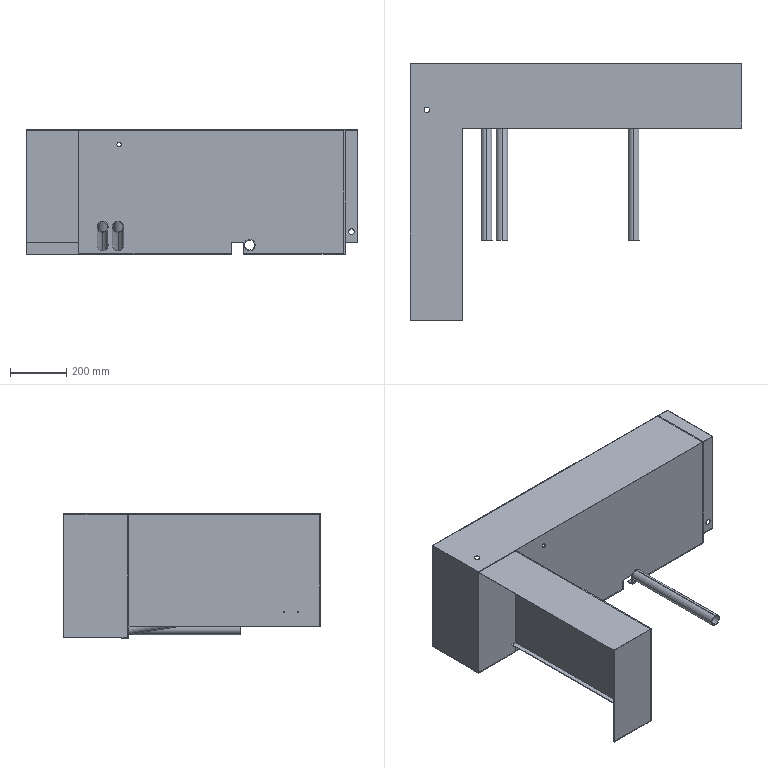Part | 6 solids | 95 faces | box 1185 x 916 x 443 mm | volume 3683413 mm3 | plane 51 | cylinder 36 | spline 8 | commonest cylinder face diameters 8 x14 40 x8 20 x6 4.2 x4 15 x2 36 x2